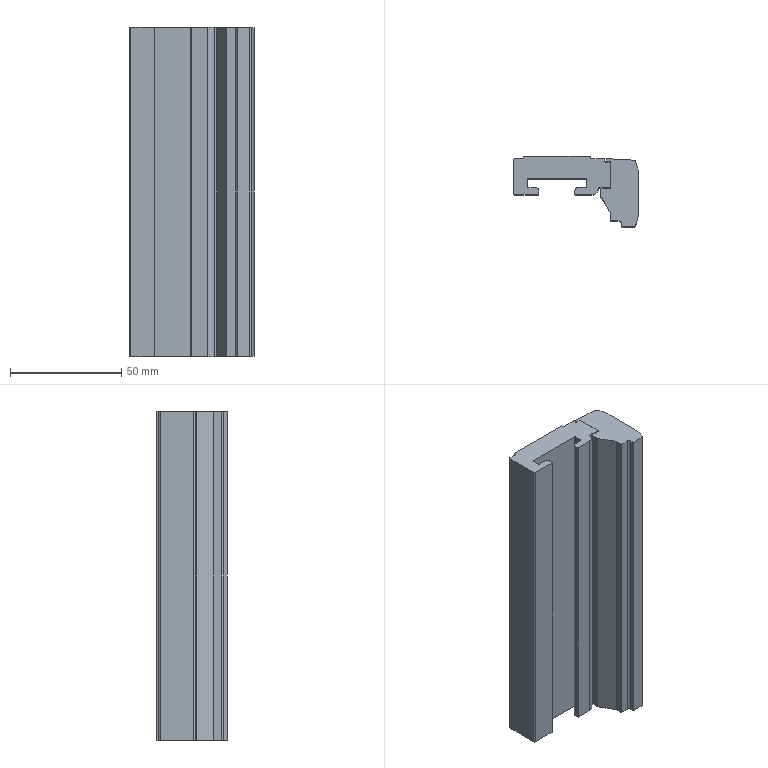Part | STEP file | DGC-25-G slider | 1 solid | 90 faces | box 56 x 31.65 x 148 mm | volume 138361 mm3 | plane 39 | cylinder 35 | cone 16 | commonest cylinder face diameters 4.134 x8 0.4 x7 0.6 x4 1 x4 3 x4 2 x3